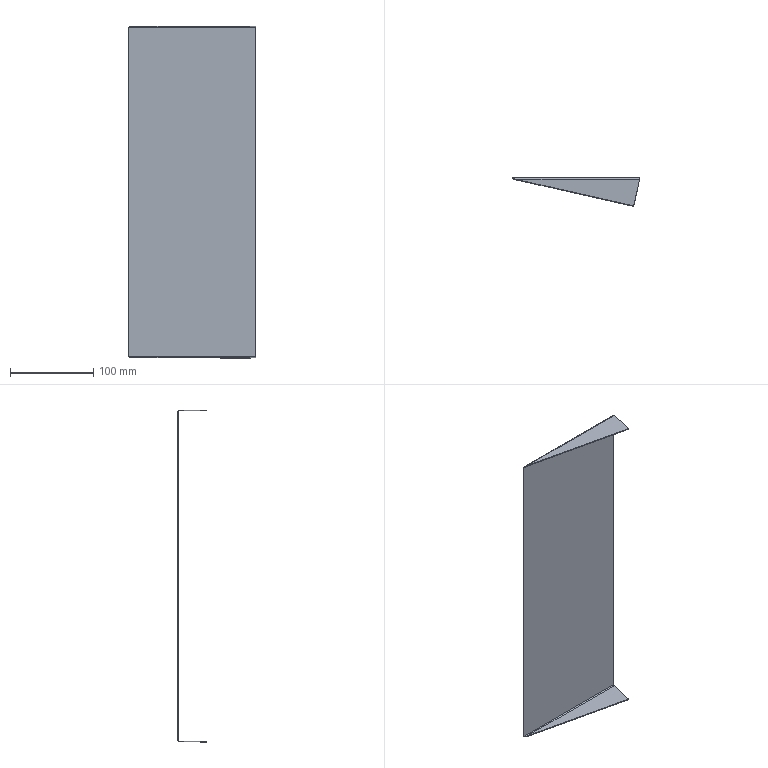Part | SolidWorks | features EdgeFlange 1, FlatPattern 1, MirrorPattern 1, SMBaseFlange 1, SheetMetal 1 | 1 solid | 20 faces | box 153.5 x 34 x 399 mm | volume 66108 mm3 | plane 12 | spline 4 | cylinder 4 | commonest cylinder face diameters 2 x2 4 x2
STEP:
#1=CARTESIAN_POINT('',(0.,-1.,-197.5));
#2=VERTEX_POINT('',#1);
#3=CARTESIAN_POINT('',(-153.5,-1.,-197.5));
#4=VERTEX_POINT('',#3);
#5=CARTESIAN_POINT('',(0.,-1.,-197.5));
#6=DIRECTION('',(-1.,0.,0.));
#7=VECTOR('',#6,1000.);
#8=LINE('',#5,#7);
#9=EDGE_CURVE('',#2,#4,#8,.T.);
#10=ORIENTED_EDGE('',*,*,#9,.F.);
#11=CARTESIAN_POINT('',(0.,-1.,197.5));
#12=VERTEX_POINT('',#11);
#13=CARTESIAN_POINT('',(0.,-1.,199.5));
#14=DIRECTION('',(0.,0.,-1.));
#15=VECTOR('',#14,1000.);
#16=LINE('',#13,#15);
#17=EDGE_CURVE('',#12,#2,#16,.T.);
#18=ORIENTED_EDGE('',*,*,#17,.F.);
#19=CARTESIAN_POINT('',(-153.5,-1.,197.5));
#20=VERTEX_POINT('',#19);
#21=CARTESIAN_POINT('',(-153.5,-1.,197.5));
#22=DIRECTION('',(1.,0.,0.));
#23=VECTOR('',#22,1000.);
#24=LINE('',#21,#23);
#25=EDGE_CURVE('',#20,#12,#24,.T.);
#26=ORIENTED_EDGE('',*,*,#25,.F.);
#27=CARTESIAN_POINT('',(-153.5,-1.,199.5));
#28=DIRECTION('',(0.,0.,-1.));
#29=VECTOR('',#28,1000.);
#30=LINE('',#27,#29);
#31=EDGE_CURVE('',#20,#4,#30,.T.);
#32=ORIENTED_EDGE('',*,*,#31,.T.);
#33=EDGE_LOOP('',(#10,#18,#26,#32));
#34=FACE_OUTER_BOUND('',#33,.T.);
#35=CARTESIAN_POINT('',(-153.5,-1.,199.5));
#36=DIRECTION('',(0.,1.,0.));
#37=DIRECTION('',(0.,0.,1.));
#38=AXIS2_PLACEMENT_3D('',#35,#36,#37);
#39=PLANE('',#38);
#40=ADVANCED_FACE('',(#34),#39,.F.);
#41=CARTESIAN_POINT('',(0.,0.,197.5));
#42=VERTEX_POINT('',#41);
#43=CARTESIAN_POINT('',(0.,0.,-197.5));
#44=VERTEX_POINT('',#43);
#45=CARTESIAN_POINT('',(0.,0.,199.5));
#46=DIRECTION('',(0.,0.,-1.));
#47=VECTOR('',#46,1000.);
#48=LINE('',#45,#47);
#49=EDGE_CURVE('',#42,#44,#48,.T.);
#50=ORIENTED_EDGE('',*,*,#49,.T.);
#51=CARTESIAN_POINT('',(-153.5,0.,-197.5));
#52=VERTEX_POINT('',#51);
#53=CARTESIAN_POINT('',(0.,0.,-197.5));
#54=DIRECTION('',(-1.,0.,0.));
#55=VECTOR('',#54,1000.);
#56=LINE('',#53,#55);
#57=EDGE_CURVE('',#44,#52,#56,.T.);
#58=ORIENTED_EDGE('',*,*,#57,.T.);
#59=CARTESIAN_POINT('',(-153.5,0.,197.5));
#60=VERTEX_POINT('',#59);
#61=CARTESIAN_POINT('',(-153.5,0.,199.5));
#62=DIRECTION('',(0.,0.,-1.));
#63=VECTOR('',#62,1000.);
#64=LINE('',#61,#63);
#65=EDGE_CURVE('',#60,#52,#64,.T.);
#66=ORIENTED_EDGE('',*,*,#65,.F.);
#67=CARTESIAN_POINT('',(-153.5,0.,197.5));
#68=DIRECTION('',(1.,0.,0.));
#69=VECTOR('',#68,1000.);
#70=LINE('',#67,#69);
#71=EDGE_CURVE('',#60,#42,#70,.T.);
#72=ORIENTED_EDGE('',*,*,#71,.T.);
#73=EDGE_LOOP('',(#50,#58,#66,#72));
#74=FACE_OUTER_BOUND('',#73,.T.);
#75=CARTESIAN_POINT('',(-153.5,0.,199.5));
#76=DIRECTION('',(0.,1.,0.));
#77=DIRECTION('',(0.,0.,1.));
#78=AXIS2_PLACEMENT_3D('',#75,#76,#77);
#79=PLANE('',#78);
#80=ADVANCED_FACE('',(#74),#79,.T.);
#81=ORIENTED_EDGE('',*,*,#17,.T.);
#82=CARTESIAN_POINT('',(0.,-1.,-197.5));
#83=DIRECTION('',(0.,1.,0.));
#84=VECTOR('',#83,1000.);
#85=LINE('',#82,#84);
#86=EDGE_CURVE('',#2,#44,#85,.T.);
#87=ORIENTED_EDGE('',*,*,#86,.T.);
#88=ORIENTED_EDGE('',*,*,#49,.F.);
#89=CARTESIAN_POINT('',(0.,-1.,197.5));
#90=DIRECTION('',(0.,1.,0.));
#91=VECTOR('',#90,1000.);
#92=LINE('',#89,#91);
#93=EDGE_CURVE('',#12,#42,#92,.T.);
#94=ORIENTED_EDGE('',*,*,#93,.F.);
#95=EDGE_LOOP('',(#81,#87,#88,#94));
#96=FACE_OUTER_BOUND('',#95,.T.);
#97=CARTESIAN_POINT('',(0.,0.,199.5));
#98=DIRECTION('',(1.,0.,0.));
#99=DIRECTION('',(0.,0.,-1.));
#100=AXIS2_PLACEMENT_3D('',#97,#98,#99);
#101=PLANE('',#100);
#102=ADVANCED_FACE('',(#96),#101,.T.);
#103=CARTESIAN_POINT('',(-153.5,-1.,-197.5));
#104=DIRECTION('',(0.,1.,0.));
#105=VECTOR('',#104,1000.);
#106=LINE('',#103,#105);
#107=EDGE_CURVE('',#4,#52,#106,.T.);
#108=ORIENTED_EDGE('',*,*,#107,.F.);
#109=ORIENTED_EDGE('',*,*,#31,.F.);
#110=CARTESIAN_POINT('',(-153.5,-1.,197.5));
#111=DIRECTION('',(0.,1.,0.));
#112=VECTOR('',#111,1000.);
#113=LINE('',#110,#112);
#114=EDGE_CURVE('',#20,#60,#113,.T.);
#115=ORIENTED_EDGE('',*,*,#114,.T.);
#116=ORIENTED_EDGE('',*,*,#65,.T.);
#117=EDGE_LOOP('',(#108,#109,#115,#116));
#118=FACE_OUTER_BOUND('',#117,.T.);
#119=CARTESIAN_POINT('',(-153.5,-1.,199.5));
#120=DIRECTION('',(-1.,0.,0.));
#121=DIRECTION('',(0.,0.,1.));
#122=AXIS2_PLACEMENT_3D('',#119,#120,#121);
#123=PLANE('',#122);
#124=ADVANCED_FACE('',(#118),#123,.T.);
#125=CARTESIAN_POINT('',(-0.226,-2.,198.5));
#126=VERTEX_POINT('',#125);
#127=CARTESIAN_POINT('',(-0.226,-2.,199.5));
#128=VERTEX_POINT('',#127);
#129=CARTESIAN_POINT('',(-0.226,-2.,199.5));
#130=DIRECTION('',(0.,0.,1.));
#131=VECTOR('',#130,1000.);
#132=LINE('',#129,#131);
#133=EDGE_CURVE('',#126,#128,#132,.T.);
#134=ORIENTED_EDGE('',*,*,#133,.F.);
#135=CARTESIAN_POINT('',(0.,-1.,197.5));
#136=CARTESIAN_POINT('',(-0.03766,-1.,197.762));
#137=CARTESIAN_POINT('',(-0.07532,-1.108,198.022));
#138=CARTESIAN_POINT('',(-0.1506,-1.478,198.392));
#139=CARTESIAN_POINT('',(-0.1883,-1.738,198.5));
#140=CARTESIAN_POINT('',(-0.226,-2.,198.5));
#141=B_SPLINE_CURVE_WITH_KNOTS('',3,(#135,#136,#137,#138,#139,#140),.UNSPECIFIED.,.F.,.F.,(4,2,4),(0.,0.5,1.),.UNSPECIFIED.);
#142=EDGE_CURVE('',#12,#126,#141,.T.);
#143=ORIENTED_EDGE('',*,*,#142,.F.);
#144=ORIENTED_EDGE('',*,*,#93,.T.);
#145=CARTESIAN_POINT('',(0.,0.,197.5));
#146=CARTESIAN_POINT('',(-0.01883,0.,197.762));
#147=CARTESIAN_POINT('',(-0.03766,-0.05205,198.023));
#148=CARTESIAN_POINT('',(-0.07532,-0.2524,198.507));
#149=CARTESIAN_POINT('',(-0.09415,-0.4007,198.729));
#150=CARTESIAN_POINT('',(-0.1318,-0.7709,199.099));
#151=CARTESIAN_POINT('',(-0.1506,-0.9928,199.248));
#152=CARTESIAN_POINT('',(-0.1883,-1.477,199.448));
#153=CARTESIAN_POINT('',(-0.2071,-1.738,199.5));
#154=CARTESIAN_POINT('',(-0.226,-2.,199.5));
#155=B_SPLINE_CURVE_WITH_KNOTS('',3,(#145,#146,#147,#148,#149,#150,#151,#152,#153,#154),.UNSPECIFIED.,.F.,.F.,(4,2,2,2,4),(0.,0.25,0.5,0.75,1.),.UNSPECIFIED.);
#156=EDGE_CURVE('',#42,#128,#155,.T.);
#157=ORIENTED_EDGE('',*,*,#156,.T.);
#158=EDGE_LOOP('',(#134,#143,#144,#157));
#159=FACE_OUTER_BOUND('',#158,.T.);
#160=CARTESIAN_POINT('',(0.,0.01,197.5));
#161=CARTESIAN_POINT('',(-0.01883,0.01,197.763));
#162=CARTESIAN_POINT('',(-0.03766,-0.04231,198.026));
#163=CARTESIAN_POINT('',(-0.07532,-0.2437,198.512));
#164=CARTESIAN_POINT('',(-0.09415,-0.3927,198.735));
#165=CARTESIAN_POINT('',(-0.1318,-0.7648,199.107));
#166=CARTESIAN_POINT('',(-0.1506,-0.9877,199.256));
#167=CARTESIAN_POINT('',(-0.1883,-1.474,199.458));
#168=CARTESIAN_POINT('',(-0.2071,-1.737,199.51));
#169=CARTESIAN_POINT('',(-0.226,-2.,199.51));
#170=CARTESIAN_POINT('',(0.,0.,197.5));
#171=CARTESIAN_POINT('',(-0.01883,0.,197.762));
#172=CARTESIAN_POINT('',(-0.03766,-0.05205,198.023));
#173=CARTESIAN_POINT('',(-0.07532,-0.2524,198.507));
#174=CARTESIAN_POINT('',(-0.09415,-0.4007,198.729));
#175=CARTESIAN_POINT('',(-0.1318,-0.7709,199.099));
#176=CARTESIAN_POINT('',(-0.1506,-0.9928,199.248));
#177=CARTESIAN_POINT('',(-0.1883,-1.477,199.448));
#178=CARTESIAN_POINT('',(-0.2071,-1.738,199.5));
#179=CARTESIAN_POINT('',(-0.226,-2.,199.5));
#180=CARTESIAN_POINT('',(0.,-1.,197.5));
#181=CARTESIAN_POINT('',(-0.01883,-1.,197.631));
#182=CARTESIAN_POINT('',(-0.03766,-1.026,197.762));
#183=CARTESIAN_POINT('',(-0.07532,-1.126,198.004));
#184=CARTESIAN_POINT('',(-0.09415,-1.2,198.115));
#185=CARTESIAN_POINT('',(-0.1318,-1.385,198.3));
#186=CARTESIAN_POINT('',(-0.1506,-1.496,198.374));
#187=CARTESIAN_POINT('',(-0.1883,-1.738,198.474));
#188=CARTESIAN_POINT('',(-0.2071,-1.869,198.5));
#189=CARTESIAN_POINT('',(-0.226,-2.,198.5));
#190=CARTESIAN_POINT('',(0.,-1.01,197.5));
#191=CARTESIAN_POINT('',(-0.01883,-1.01,197.63));
#192=CARTESIAN_POINT('',(-0.03766,-1.036,197.759));
#193=CARTESIAN_POINT('',(-0.07532,-1.135,197.999));
#194=CARTESIAN_POINT('',(-0.09415,-1.208,198.108));
#195=CARTESIAN_POINT('',(-0.1318,-1.392,198.292));
#196=CARTESIAN_POINT('',(-0.1506,-1.501,198.365));
#197=CARTESIAN_POINT('',(-0.1883,-1.741,198.464));
#198=CARTESIAN_POINT('',(-0.2071,-1.87,198.49));
#199=CARTESIAN_POINT('',(-0.226,-2.,198.49));
#200=B_SPLINE_SURFACE_WITH_KNOTS('',1,3,((#160,#161,#162,#163,#164,#165,#166,#167,#168,#169),(#170,#171,#172,#173,#174,#175,#176,#177,#178,#179),(#180,#181,#182,#183,#184,#185,#186,#187,#188,#189),(#190,#191,#192,#193,#194,#195,#196,#197,#198,#199)),.UNSPECIFIED.,.F.,.F.,.F.,(2,1,1,2),(4,2,2,2,4),(-0.01,0.,1.,1.01),(0.,0.25,0.5,0.75,1.),.UNSPECIFIED.);
#201=ADVANCED_FACE('',(#159),#200,.F.);
#202=CARTESIAN_POINT('',(-149.074,-2.,198.5));
#203=VERTEX_POINT('',#202);
#204=CARTESIAN_POINT('',(-149.074,-2.,198.5));
#205=CARTESIAN_POINT('',(-149.444,-1.869,198.5));
#206=CARTESIAN_POINT('',(-149.811,-1.738,198.474));
#207=CARTESIAN_POINT('',(-150.547,-1.497,198.374));
#208=CARTESIAN_POINT('',(-150.916,-1.386,198.3));
#209=CARTESIAN_POINT('',(-151.654,-1.201,198.115));
#210=CARTESIAN_POINT('',(-152.023,-1.126,198.004));
#211=CARTESIAN_POINT('',(-152.762,-1.026,197.762));
#212=CARTESIAN_POINT('',(-153.13,-1.,197.631));
#213=CARTESIAN_POINT('',(-153.5,-1.,197.5));
#214=B_SPLINE_CURVE_WITH_KNOTS('',3,(#204,#205,#206,#207,#208,#209,#210,#211,#212,#213),.UNSPECIFIED.,.F.,.F.,(4,2,2,2,4),(0.,0.00117,0.00234,0.00351,0.00468),.UNSPECIFIED.);
#215=EDGE_CURVE('',#203,#20,#214,.T.);
#216=ORIENTED_EDGE('',*,*,#215,.F.);
#217=CARTESIAN_POINT('',(-149.074,-2.,199.5));
#218=VERTEX_POINT('',#217);
#219=CARTESIAN_POINT('',(-149.074,-2.,198.5));
#220=DIRECTION('',(0.,0.,1.));
#221=VECTOR('',#220,1000.);
#222=LINE('',#219,#221);
#223=EDGE_CURVE('',#203,#218,#222,.T.);
#224=ORIENTED_EDGE('',*,*,#223,.T.);
#225=CARTESIAN_POINT('',(-149.074,-2.,199.5));
#226=CARTESIAN_POINT('',(-149.446,-1.736,199.5));
#227=CARTESIAN_POINT('',(-149.811,-1.477,199.448));
#228=CARTESIAN_POINT('',(-150.545,-0.9954,199.249));
#229=CARTESIAN_POINT('',(-150.918,-0.771,199.099));
#230=CARTESIAN_POINT('',(-151.653,-0.4023,198.731));
#231=CARTESIAN_POINT('',(-152.018,-0.2546,198.512));
#232=CARTESIAN_POINT('',(-152.761,-0.05202,198.024));
#233=CARTESIAN_POINT('',(-153.128,0.,197.764));
#234=CARTESIAN_POINT('',(-153.5,0.,197.5));
#235=B_SPLINE_CURVE_WITH_KNOTS('',3,(#225,#226,#227,#228,#229,#230,#231,#232,#233,#234),.UNSPECIFIED.,.F.,.F.,(4,2,2,2,4),(0.,0.001349,0.002697,0.004046,0.005395),.UNSPECIFIED.);
#236=EDGE_CURVE('',#218,#60,#235,.T.);
#237=ORIENTED_EDGE('',*,*,#236,.T.);
#238=ORIENTED_EDGE('',*,*,#114,.F.);
#239=EDGE_LOOP('',(#216,#224,#237,#238));
#240=FACE_OUTER_BOUND('',#239,.T.);
#241=CARTESIAN_POINT('',(-149.074,-2.,199.51));
#242=CARTESIAN_POINT('',(-149.443,-1.737,199.51));
#243=CARTESIAN_POINT('',(-149.812,-1.474,199.458));
#244=CARTESIAN_POINT('',(-150.55,-0.9877,199.256));
#245=CARTESIAN_POINT('',(-150.918,-0.7648,199.107));
#246=CARTESIAN_POINT('',(-151.656,-0.3927,198.735));
#247=CARTESIAN_POINT('',(-152.025,-0.2437,198.512));
#248=CARTESIAN_POINT('',(-152.762,-0.04231,198.026));
#249=CARTESIAN_POINT('',(-153.131,0.01,197.763));
#250=CARTESIAN_POINT('',(-153.5,0.01,197.5));
#251=CARTESIAN_POINT('',(-149.074,-2.,199.5));
#252=CARTESIAN_POINT('',(-149.443,-1.738,199.5));
#253=CARTESIAN_POINT('',(-149.812,-1.477,199.448));
#254=CARTESIAN_POINT('',(-150.55,-0.9928,199.248));
#255=CARTESIAN_POINT('',(-150.918,-0.7709,199.099));
#256=CARTESIAN_POINT('',(-151.656,-0.4007,198.729));
#257=CARTESIAN_POINT('',(-152.025,-0.2524,198.507));
#258=CARTESIAN_POINT('',(-152.762,-0.05205,198.023));
#259=CARTESIAN_POINT('',(-153.131,0.,197.762));
#260=CARTESIAN_POINT('',(-153.5,0.,197.5));
#261=CARTESIAN_POINT('',(-149.074,-2.,198.5));
#262=CARTESIAN_POINT('',(-149.443,-1.869,198.5));
#263=CARTESIAN_POINT('',(-149.812,-1.738,198.474));
#264=CARTESIAN_POINT('',(-150.55,-1.496,198.374));
#265=CARTESIAN_POINT('',(-150.918,-1.385,198.3));
#266=CARTESIAN_POINT('',(-151.656,-1.2,198.115));
#267=CARTESIAN_POINT('',(-152.025,-1.126,198.004));
#268=CARTESIAN_POINT('',(-152.762,-1.026,197.762));
#269=CARTESIAN_POINT('',(-153.131,-1.,197.631));
#270=CARTESIAN_POINT('',(-153.5,-1.,197.5));
#271=CARTESIAN_POINT('',(-149.074,-2.,198.49));
#272=CARTESIAN_POINT('',(-149.443,-1.87,198.49));
#273=CARTESIAN_POINT('',(-149.812,-1.741,198.464));
#274=CARTESIAN_POINT('',(-150.55,-1.501,198.365));
#275=CARTESIAN_POINT('',(-150.918,-1.392,198.292));
#276=CARTESIAN_POINT('',(-151.656,-1.208,198.108));
#277=CARTESIAN_POINT('',(-152.025,-1.135,197.999));
#278=CARTESIAN_POINT('',(-152.762,-1.036,197.759));
#279=CARTESIAN_POINT('',(-153.131,-1.01,197.63));
#280=CARTESIAN_POINT('',(-153.5,-1.01,197.5));
#281=B_SPLINE_SURFACE_WITH_KNOTS('',1,3,((#241,#242,#243,#244,#245,#246,#247,#248,#249,#250),(#251,#252,#253,#254,#255,#256,#257,#258,#259,#260),(#261,#262,#263,#264,#265,#266,#267,#268,#269,#270),(#271,#272,#273,#274,#275,#276,#277,#278,#279,#280)),.UNSPECIFIED.,.F.,.F.,.F.,(2,1,1,2),(4,2,2,2,4),(-0.01,0.,1.,1.01),(0.,0.25,0.5,0.75,1.),.UNSPECIFIED.);
#282=ADVANCED_FACE('',(#240),#281,.F.);
#283=ORIENTED_EDGE('',*,*,#71,.F.);
#284=ORIENTED_EDGE('',*,*,#236,.F.);
#285=CARTESIAN_POINT('',(-0.226,-2.,199.5));
#286=DIRECTION('',(1.,0.,0.));
#287=VECTOR('',#286,1000.);
#288=LINE('',#285,#287);
#289=EDGE_CURVE('',#218,#128,#288,.T.);
#290=ORIENTED_EDGE('',*,*,#289,.T.);
#291=ORIENTED_EDGE('',*,*,#156,.F.);
#292=EDGE_LOOP('',(#283,#284,#290,#291));
#293=FACE_OUTER_BOUND('',#292,.T.);
#294=CARTESIAN_POINT('',(-153.5,-2.,197.5));
#295=DIRECTION('',(-1.,0.,0.));
#296=DIRECTION('',(0.,0.,1.));
#297=AXIS2_PLACEMENT_3D('',#294,#295,#296);
#298=CYLINDRICAL_SURFACE('',#297,2.);
#299=ADVANCED_FACE('',(#293),#298,.T.);
#300=ORIENTED_EDGE('',*,*,#25,.T.);
#301=ORIENTED_EDGE('',*,*,#142,.T.);
#302=CARTESIAN_POINT('',(-0.226,-2.,198.5));
#303=DIRECTION('',(-1.,0.,0.));
#304=VECTOR('',#303,1000.);
#305=LINE('',#302,#304);
#306=EDGE_CURVE('',#126,#203,#305,.T.);
#307=ORIENTED_EDGE('',*,*,#306,.T.);
#308=ORIENTED_EDGE('',*,*,#215,.T.);
#309=EDGE_LOOP('',(#300,#301,#307,#308));
#310=FACE_OUTER_BOUND('',#309,.T.);
#311=CARTESIAN_POINT('',(-153.5,-2.,197.5));
#312=DIRECTION('',(-1.,0.,0.));
#313=DIRECTION('',(0.,0.,1.));
#314=AXIS2_PLACEMENT_3D('',#311,#312,#313);
#315=CYLINDRICAL_SURFACE('',#314,1.);
#316=ADVANCED_FACE('',(#310),#315,.F.);
#317=CARTESIAN_POINT('',(-7.457,-34.,199.5));
#318=VERTEX_POINT('',#317);
#319=CARTESIAN_POINT('',(-153.5,-1.,199.5));
#320=DIRECTION('',(-0.9754,0.2204,0.));
#321=VECTOR('',#320,1000.);
#322=LINE('',#319,#321);
#323=EDGE_CURVE('',#318,#218,#322,.T.);
#324=ORIENTED_EDGE('',*,*,#323,.T.);
#325=ORIENTED_EDGE('',*,*,#223,.F.);
#326=CARTESIAN_POINT('',(-7.457,-34.,198.5));
#327=VERTEX_POINT('',#326);
#328=CARTESIAN_POINT('',(-7.672,-33.951,198.5));
#329=DIRECTION('',(-0.9754,0.2204,0.));
#330=VECTOR('',#329,1000.);
#331=LINE('',#328,#330);
#332=EDGE_CURVE('',#327,#203,#331,.T.);
#333=ORIENTED_EDGE('',*,*,#332,.F.);
#334=CARTESIAN_POINT('',(-7.457,-34.,199.5));
#335=DIRECTION('',(0.,0.,-1.));
#336=VECTOR('',#335,1000.);
#337=LINE('',#334,#336);
#338=EDGE_CURVE('',#318,#327,#337,.T.);
#339=ORIENTED_EDGE('',*,*,#338,.F.);
#340=EDGE_LOOP('',(#324,#325,#333,#339));
#341=FACE_OUTER_BOUND('',#340,.T.);
#342=CARTESIAN_POINT('',(-153.5,-1.,199.5));
#343=DIRECTION('',(-0.2204,-0.9754,0.));
#344=DIRECTION('',(0.9754,-0.2204,0.));
#345=AXIS2_PLACEMENT_3D('',#342,#343,#344);
#346=PLANE('',#345);
#347=ADVANCED_FACE('',(#341),#346,.T.);
#348=CARTESIAN_POINT('',(0.215,-0.04858,198.5));
#349=DIRECTION('',(-0.2204,-0.9754,0.));
#350=VECTOR('',#349,1000.);
#351=LINE('',#348,#350);
#352=EDGE_CURVE('',#126,#327,#351,.T.);
#353=ORIENTED_EDGE('',*,*,#352,.F.);
#354=ORIENTED_EDGE('',*,*,#133,.T.);
#355=CARTESIAN_POINT('',(-7.457,-34.,199.5));
#356=DIRECTION('',(-0.2204,-0.9754,0.));
#357=VECTOR('',#356,1000.);
#358=LINE('',#355,#357);
#359=EDGE_CURVE('',#128,#318,#358,.T.);
#360=ORIENTED_EDGE('',*,*,#359,.T.);
#361=ORIENTED_EDGE('',*,*,#338,.T.);
#362=EDGE_LOOP('',(#353,#354,#360,#361));
#363=FACE_OUTER_BOUND('',#362,.T.);
#364=CARTESIAN_POINT('',(-7.457,-34.,199.5));
#365=DIRECTION('',(0.9754,-0.2204,0.));
#366=DIRECTION('',(0.2204,0.9754,0.));
#367=AXIS2_PLACEMENT_3D('',#364,#365,#366);
#368=PLANE('',#367);
#369=ADVANCED_FACE('',(#363),#368,.T.);
#370=ORIENTED_EDGE('',*,*,#289,.F.);
#371=ORIENTED_EDGE('',*,*,#323,.F.);
#372=ORIENTED_EDGE('',*,*,#359,.F.);
#373=EDGE_LOOP('',(#370,#371,#372));
#374=FACE_OUTER_BOUND('',#373,.T.);
#375=CARTESIAN_POINT('',(0.,0.,199.5));
#376=DIRECTION('',(0.,0.,-1.));
#377=DIRECTION('',(0.,1.,0.));
#378=AXIS2_PLACEMENT_3D('',#375,#376,#377);
#379=PLANE('',#378);
#380=ADVANCED_FACE('',(#374),#379,.F.);
#381=ORIENTED_EDGE('',*,*,#332,.T.);
#382=ORIENTED_EDGE('',*,*,#306,.F.);
#383=ORIENTED_EDGE('',*,*,#352,.T.);
#384=EDGE_LOOP('',(#381,#382,#383));
#385=FACE_OUTER_BOUND('',#384,.T.);
#386=CARTESIAN_POINT('',(0.,0.,198.5));
#387=DIRECTION('',(0.,0.,-1.));
#388=DIRECTION('',(0.,1.,0.));
#389=AXIS2_PLACEMENT_3D('',#386,#387,#388);
#390=PLANE('',#389);
#391=ADVANCED_FACE('',(#385),#390,.T.);
#392=CARTESIAN_POINT('',(-149.074,-2.,-198.5));
#393=VERTEX_POINT('',#392);
#394=CARTESIAN_POINT('',(-149.074,-2.,-199.5));
#395=VERTEX_POINT('',#394);
#396=CARTESIAN_POINT('',(-149.074,-2.,-199.5));
#397=DIRECTION('',(0.,0.,-1.));
#398=VECTOR('',#397,1000.);
#399=LINE('',#396,#398);
#400=EDGE_CURVE('',#393,#395,#399,.T.);
#401=ORIENTED_EDGE('',*,*,#400,.F.);
#402=CARTESIAN_POINT('',(-153.5,-1.,-197.5));
#403=CARTESIAN_POINT('',(-153.13,-1.,-197.631));
#404=CARTESIAN_POINT('',(-152.763,-1.026,-197.762));
#405=CARTESIAN_POINT('',(-152.028,-1.126,-198.003));
#406=CARTESIAN_POINT('',(-151.658,-1.2,-198.114));
#407=CARTESIAN_POINT('',(-150.92,-1.385,-198.299));
#408=CARTESIAN_POINT('',(-150.551,-1.496,-198.374));
#409=CARTESIAN_POINT('',(-149.812,-1.738,-198.474));
#410=CARTESIAN_POINT('',(-149.444,-1.869,-198.5));
#411=CARTESIAN_POINT('',(-149.074,-2.,-198.5));
#412=B_SPLINE_CURVE_WITH_KNOTS('',3,(#402,#403,#404,#405,#406,#407,#408,#409,#410,#411),.UNSPECIFIED.,.F.,.F.,(4,2,2,2,4),(0.,0.00117,0.00234,0.00351,0.00468),.UNSPECIFIED.);
#413=EDGE_CURVE('',#4,#393,#412,.T.);
#414=ORIENTED_EDGE('',*,*,#413,.F.);
#415=ORIENTED_EDGE('',*,*,#107,.T.);
#416=CARTESIAN_POINT('',(-153.5,0.,-197.5));
#417=CARTESIAN_POINT('',(-153.128,0.,-197.764));
#418=CARTESIAN_POINT('',(-152.763,-0.05201,-198.023));
#419=CARTESIAN_POINT('',(-152.029,-0.2511,-198.505));
#420=CARTESIAN_POINT('',(-151.656,-0.4008,-198.729));
#421=CARTESIAN_POINT('',(-150.922,-0.7691,-199.098));
#422=CARTESIAN_POINT('',(-150.556,-0.9885,-199.245));
#423=CARTESIAN_POINT('',(-149.813,-1.476,-199.448));
#424=CARTESIAN_POINT('',(-149.446,-1.736,-199.5));
#425=CARTESIAN_POINT('',(-149.074,-2.,-199.5));
#426=B_SPLINE_CURVE_WITH_KNOTS('',3,(#416,#417,#418,#419,#420,#421,#422,#423,#424,#425),.UNSPECIFIED.,.F.,.F.,(4,2,2,2,4),(0.,0.001349,0.002697,0.004046,0.005395),.UNSPECIFIED.);
#427=EDGE_CURVE('',#52,#395,#426,.T.);
#428=ORIENTED_EDGE('',*,*,#427,.T.);
#429=EDGE_LOOP('',(#401,#414,#415,#428));
#430=FACE_OUTER_BOUND('',#429,.T.);
#431=CARTESIAN_POINT('',(-153.5,0.01,-197.5));
#432=CARTESIAN_POINT('',(-153.131,0.01,-197.763));
#433=CARTESIAN_POINT('',(-152.762,-0.04231,-198.026));
#434=CARTESIAN_POINT('',(-152.025,-0.2437,-198.512));
#435=CARTESIAN_POINT('',(-151.656,-0.3927,-198.735));
#436=CARTESIAN_POINT('',(-150.918,-0.7648,-199.107));
#437=CARTESIAN_POINT('',(-150.55,-0.9877,-199.256));
#438=CARTESIAN_POINT('',(-149.812,-1.474,-199.458));
#439=CARTESIAN_POINT('',(-149.443,-1.737,-199.51));
#440=CARTESIAN_POINT('',(-149.074,-2.,-199.51));
#441=CARTESIAN_POINT('',(-153.5,0.,-197.5));
#442=CARTESIAN_POINT('',(-153.131,0.,-197.762));
#443=CARTESIAN_POINT('',(-152.762,-0.05205,-198.023));
#444=CARTESIAN_POINT('',(-152.025,-0.2524,-198.507));
#445=CARTESIAN_POINT('',(-151.656,-0.4007,-198.729));
#446=CARTESIAN_POINT('',(-150.918,-0.7709,-199.099));
#447=CARTESIAN_POINT('',(-150.55,-0.9928,-199.248));
#448=CARTESIAN_POINT('',(-149.812,-1.477,-199.448));
#449=CARTESIAN_POINT('',(-149.443,-1.738,-199.5));
#450=CARTESIAN_POINT('',(-149.074,-2.,-199.5));
#451=CARTESIAN_POINT('',(-153.5,-1.,-197.5));
#452=CARTESIAN_POINT('',(-153.131,-1.,-197.631));
#453=CARTESIAN_POINT('',(-152.762,-1.026,-197.762));
#454=CARTESIAN_POINT('',(-152.025,-1.126,-198.004));
#455=CARTESIAN_POINT('',(-151.656,-1.2,-198.115));
#456=CARTESIAN_POINT('',(-150.918,-1.385,-198.3));
#457=CARTESIAN_POINT('',(-150.55,-1.496,-198.374));
#458=CARTESIAN_POINT('',(-149.812,-1.738,-198.474));
#459=CARTESIAN_POINT('',(-149.443,-1.869,-198.5));
#460=CARTESIAN_POINT('',(-149.074,-2.,-198.5));
#461=CARTESIAN_POINT('',(-153.5,-1.01,-197.5));
#462=CARTESIAN_POINT('',(-153.131,-1.01,-197.63));
#463=CARTESIAN_POINT('',(-152.762,-1.036,-197.759));
#464=CARTESIAN_POINT('',(-152.025,-1.135,-197.999));
#465=CARTESIAN_POINT('',(-151.656,-1.208,-198.108));
#466=CARTESIAN_POINT('',(-150.918,-1.392,-198.292));
#467=CARTESIAN_POINT('',(-150.55,-1.501,-198.365));
#468=CARTESIAN_POINT('',(-149.812,-1.741,-198.464));
#469=CARTESIAN_POINT('',(-149.443,-1.87,-198.49));
#470=CARTESIAN_POINT('',(-149.074,-2.,-198.49));
#471=B_SPLINE_SURFACE_WITH_KNOTS('',1,3,((#431,#432,#433,#434,#435,#436,#437,#438,#439,#440),(#441,#442,#443,#444,#445,#446,#447,#448,#449,#450),(#451,#452,#453,#454,#455,#456,#457,#458,#459,#460),(#461,#462,#463,#464,#465,#466,#467,#468,#469,#470)),.UNSPECIFIED.,.F.,.F.,.F.,(2,1,1,2),(4,2,2,2,4),(-0.01,0.,1.,1.01),(0.,0.25,0.5,0.75,1.),.UNSPECIFIED.);
#472=ADVANCED_FACE('',(#430),#471,.F.);
#473=CARTESIAN_POINT('',(-0.226,-2.,-198.5));
#474=VERTEX_POINT('',#473);
#475=CARTESIAN_POINT('',(-0.226,-2.,-198.5));
#476=CARTESIAN_POINT('',(-0.1883,-1.738,-198.5));
#477=CARTESIAN_POINT('',(-0.1506,-1.478,-198.392));
#478=CARTESIAN_POINT('',(-0.07532,-1.108,-198.022));
#479=CARTESIAN_POINT('',(-0.03766,-1.,-197.762));
#480=CARTESIAN_POINT('',(0.,-1.,-197.5));
#481=B_SPLINE_CURVE_WITH_KNOTS('',3,(#475,#476,#477,#478,#479,#480),.UNSPECIFIED.,.F.,.F.,(4,2,4),(0.,0.5,1.),.UNSPECIFIED.);
#482=EDGE_CURVE('',#474,#2,#481,.T.);
#483=ORIENTED_EDGE('',*,*,#482,.F.);
#484=CARTESIAN_POINT('',(-0.226,-2.,-199.5));
#485=VERTEX_POINT('',#484);
#486=CARTESIAN_POINT('',(-0.226,-2.,-198.5));
#487=DIRECTION('',(0.,0.,-1.));
#488=VECTOR('',#487,1000.);
#489=LINE('',#486,#488);
#490=EDGE_CURVE('',#474,#485,#489,.T.);
#491=ORIENTED_EDGE('',*,*,#490,.T.);
#492=CARTESIAN_POINT('',(-0.226,-2.,-199.5));
#493=CARTESIAN_POINT('',(-0.2071,-1.738,-199.5));
#494=CARTESIAN_POINT('',(-0.1883,-1.477,-199.448));
#495=CARTESIAN_POINT('',(-0.1506,-0.9928,-199.248));
#496=CARTESIAN_POINT('',(-0.1318,-0.7709,-199.099));
#497=CARTESIAN_POINT('',(-0.09415,-0.4007,-198.729));
#498=CARTESIAN_POINT('',(-0.07532,-0.2524,-198.507));
#499=CARTESIAN_POINT('',(-0.03766,-0.05205,-198.023));
#500=CARTESIAN_POINT('',(-0.01883,0.,-197.762));
#501=CARTESIAN_POINT('',(0.,0.,-197.5));
#502=B_SPLINE_CURVE_WITH_KNOTS('',3,(#492,#493,#494,#495,#496,#497,#498,#499,#500,#501),.UNSPECIFIED.,.F.,.F.,(4,2,2,2,4),(0.,0.25,0.5,0.75,1.),.UNSPECIFIED.);
#503=EDGE_CURVE('',#485,#44,#502,.T.);
#504=ORIENTED_EDGE('',*,*,#503,.T.);
#505=ORIENTED_EDGE('',*,*,#86,.F.);
#506=EDGE_LOOP('',(#483,#491,#504,#505));
#507=FACE_OUTER_BOUND('',#506,.T.);
#508=CARTESIAN_POINT('',(-0.226,-2.,-199.51));
#509=CARTESIAN_POINT('',(-0.2071,-1.737,-199.51));
#510=CARTESIAN_POINT('',(-0.1883,-1.474,-199.458));
#511=CARTESIAN_POINT('',(-0.1506,-0.9877,-199.256));
#512=CARTESIAN_POINT('',(-0.1318,-0.7648,-199.107));
#513=CARTESIAN_POINT('',(-0.09415,-0.3927,-198.735));
#514=CARTESIAN_POINT('',(-0.07532,-0.2437,-198.512));
#515=CARTESIAN_POINT('',(-0.03766,-0.04231,-198.026));
#516=CARTESIAN_POINT('',(-0.01883,0.01,-197.763));
#517=CARTESIAN_POINT('',(0.,0.01,-197.5));
#518=CARTESIAN_POINT('',(-0.226,-2.,-199.5));
#519=CARTESIAN_POINT('',(-0.2071,-1.738,-199.5));
#520=CARTESIAN_POINT('',(-0.1883,-1.477,-199.448));
#521=CARTESIAN_POINT('',(-0.1506,-0.9928,-199.248));
#522=CARTESIAN_POINT('',(-0.1318,-0.7709,-199.099));
#523=CARTESIAN_POINT('',(-0.09415,-0.4007,-198.729));
#524=CARTESIAN_POINT('',(-0.07532,-0.2524,-198.507));
#525=CARTESIAN_POINT('',(-0.03766,-0.05205,-198.023));
#526=CARTESIAN_POINT('',(-0.01883,0.,-197.762));
#527=CARTESIAN_POINT('',(0.,0.,-197.5));
#528=CARTESIAN_POINT('',(-0.226,-2.,-198.5));
#529=CARTESIAN_POINT('',(-0.2071,-1.869,-198.5));
#530=CARTESIAN_POINT('',(-0.1883,-1.738,-198.474));
#531=CARTESIAN_POINT('',(-0.1506,-1.496,-198.374));
#532=CARTESIAN_POINT('',(-0.1318,-1.385,-198.3));
#533=CARTESIAN_POINT('',(-0.09415,-1.2,-198.115));
#534=CARTESIAN_POINT('',(-0.07532,-1.126,-198.004));
#535=CARTESIAN_POINT('',(-0.03766,-1.026,-197.762));
#536=CARTESIAN_POINT('',(-0.01883,-1.,-197.631));
#537=CARTESIAN_POINT('',(0.,-1.,-197.5));
#538=CARTESIAN_POINT('',(-0.226,-2.,-198.49));
#539=CARTESIAN_POINT('',(-0.2071,-1.87,-198.49));
#540=CARTESIAN_POINT('',(-0.1883,-1.741,-198.464));
#541=CARTESIAN_POINT('',(-0.1506,-1.501,-198.365));
#542=CARTESIAN_POINT('',(-0.1318,-1.392,-198.292));
#543=CARTESIAN_POINT('',(-0.09415,-1.208,-198.108));
#544=CARTESIAN_POINT('',(-0.07532,-1.135,-197.999));
#545=CARTESIAN_POINT('',(-0.03766,-1.036,-197.759));
#546=CARTESIAN_POINT('',(-0.01883,-1.01,-197.63));
#547=CARTESIAN_POINT('',(0.,-1.01,-197.5));
#548=B_SPLINE_SURFACE_WITH_KNOTS('',1,3,((#508,#509,#510,#511,#512,#513,#514,#515,#516,#517),(#518,#519,#520,#521,#522,#523,#524,#525,#526,#527),(#528,#529,#530,#531,#532,#533,#534,#535,#536,#537),(#538,#539,#540,#541,#542,#543,#544,#545,#546,#547)),.UNSPECIFIED.,.F.,.F.,.F.,(2,1,1,2),(4,2,2,2,4),(-0.01,0.,1.,1.01),(0.,0.25,0.5,0.75,1.),.UNSPECIFIED.);
#549=ADVANCED_FACE('',(#507),#548,.F.);
#550=ORIENTED_EDGE('',*,*,#57,.F.);
#551=ORIENTED_EDGE('',*,*,#503,.F.);
#552=CARTESIAN_POINT('',(-149.074,-2.,-199.5));
#553=DIRECTION('',(-1.,0.,0.));
#554=VECTOR('',#553,1000.);
#555=LINE('',#552,#554);
#556=EDGE_CURVE('',#485,#395,#555,.T.);
#557=ORIENTED_EDGE('',*,*,#556,.T.);
#558=ORIENTED_EDGE('',*,*,#427,.F.);
#559=EDGE_LOOP('',(#550,#551,#557,#558));
#560=FACE_OUTER_BOUND('',#559,.T.);
#561=CARTESIAN_POINT('',(0.,-2.,-197.5));
#562=DIRECTION('',(1.,0.,0.));
#563=DIRECTION('',(0.,0.,-1.));
#564=AXIS2_PLACEMENT_3D('',#561,#562,#563);
#565=CYLINDRICAL_SURFACE('',#564,2.);
#566=ADVANCED_FACE('',(#560),#565,.T.);
#567=ORIENTED_EDGE('',*,*,#9,.T.);
#568=ORIENTED_EDGE('',*,*,#413,.T.);
#569=CARTESIAN_POINT('',(-149.074,-2.,-198.5));
#570=DIRECTION('',(1.,0.,0.));
#571=VECTOR('',#570,1000.);
#572=LINE('',#569,#571);
#573=EDGE_CURVE('',#393,#474,#572,.T.);
#574=ORIENTED_EDGE('',*,*,#573,.T.);
#575=ORIENTED_EDGE('',*,*,#482,.T.);
#576=EDGE_LOOP('',(#567,#568,#574,#575));
#577=FACE_OUTER_BOUND('',#576,.T.);
#578=CARTESIAN_POINT('',(0.,-2.,-197.5));
#579=DIRECTION('',(1.,0.,0.));
#580=DIRECTION('',(0.,0.,-1.));
#581=AXIS2_PLACEMENT_3D('',#578,#579,#580);
#582=CYLINDRICAL_SURFACE('',#581,1.);
#583=ADVANCED_FACE('',(#577),#582,.F.);
#584=ORIENTED_EDGE('',*,*,#490,.F.);
#585=CARTESIAN_POINT('',(-7.457,-34.,-198.5));
#586=VERTEX_POINT('',#585);
#587=CARTESIAN_POINT('',(-7.457,-34.,-198.5));
#588=DIRECTION('',(-0.2204,-0.9754,0.));
#589=VECTOR('',#588,1000.);
#590=LINE('',#587,#589);
#591=EDGE_CURVE('',#474,#586,#590,.T.);
#592=ORIENTED_EDGE('',*,*,#591,.T.);
#593=CARTESIAN_POINT('',(-7.457,-34.,-199.5));
#594=VERTEX_POINT('',#593);
#595=CARTESIAN_POINT('',(-7.457,-34.,-199.5));
#596=DIRECTION('',(0.,0.,1.));
#597=VECTOR('',#596,1000.);
#598=LINE('',#595,#597);
#599=EDGE_CURVE('',#594,#586,#598,.T.);
#600=ORIENTED_EDGE('',*,*,#599,.F.);
#601=CARTESIAN_POINT('',(0.215,-0.04858,-199.5));
#602=DIRECTION('',(-0.2204,-0.9754,0.));
#603=VECTOR('',#602,1000.);
#604=LINE('',#601,#603);
#605=EDGE_CURVE('',#485,#594,#604,.T.);
#606=ORIENTED_EDGE('',*,*,#605,.F.);
#607=EDGE_LOOP('',(#584,#592,#600,#606));
#608=FACE_OUTER_BOUND('',#607,.T.);
#609=CARTESIAN_POINT('',(-7.457,-34.,-199.5));
#610=DIRECTION('',(-0.9754,0.2204,0.));
#611=DIRECTION('',(-0.2204,-0.9754,0.));
#612=AXIS2_PLACEMENT_3D('',#609,#610,#611);
#613=PLANE('',#612);
#614=ADVANCED_FACE('',(#608),#613,.F.);
#615=ORIENTED_EDGE('',*,*,#400,.T.);
#616=CARTESIAN_POINT('',(-7.672,-33.951,-199.5));
#617=DIRECTION('',(-0.9754,0.2204,0.));
#618=VECTOR('',#617,1000.);
#619=LINE('',#616,#618);
#620=EDGE_CURVE('',#594,#395,#619,.T.);
#621=ORIENTED_EDGE('',*,*,#620,.F.);
#622=ORIENTED_EDGE('',*,*,#599,.T.);
#623=CARTESIAN_POINT('',(-153.5,-1.,-198.5));
#624=DIRECTION('',(-0.9754,0.2204,0.));
#625=VECTOR('',#624,1000.);
#626=LINE('',#623,#625);
#627=EDGE_CURVE('',#586,#393,#626,.T.);
#628=ORIENTED_EDGE('',*,*,#627,.T.);
#629=EDGE_LOOP('',(#615,#621,#622,#628));
#630=FACE_OUTER_BOUND('',#629,.T.);
#631=CARTESIAN_POINT('',(-153.5,-1.,-199.5));
#632=DIRECTION('',(0.2204,0.9754,0.));
#633=DIRECTION('',(-0.9754,0.2204,0.));
#634=AXIS2_PLACEMENT_3D('',#631,#632,#633);
#635=PLANE('',#634);
#636=ADVANCED_FACE('',(#630),#635,.F.);
#637=ORIENTED_EDGE('',*,*,#556,.F.);
#638=ORIENTED_EDGE('',*,*,#605,.T.);
#639=ORIENTED_EDGE('',*,*,#620,.T.);
#640=EDGE_LOOP('',(#637,#638,#639));
#641=FACE_OUTER_BOUND('',#640,.T.);
#642=CARTESIAN_POINT('',(0.,0.,-199.5));
#643=DIRECTION('',(0.,0.,1.));
#644=DIRECTION('',(0.,1.,0.));
#645=AXIS2_PLACEMENT_3D('',#642,#643,#644);
#646=PLANE('',#645);
#647=ADVANCED_FACE('',(#641),#646,.F.);
#648=ORIENTED_EDGE('',*,*,#591,.F.);
#649=ORIENTED_EDGE('',*,*,#573,.F.);
#650=ORIENTED_EDGE('',*,*,#627,.F.);
#651=EDGE_LOOP('',(#648,#649,#650));
#652=FACE_OUTER_BOUND('',#651,.T.);
#653=CARTESIAN_POINT('',(0.,0.,-198.5));
#654=DIRECTION('',(0.,0.,1.));
#655=DIRECTION('',(0.,1.,0.));
#656=AXIS2_PLACEMENT_3D('',#653,#654,#655);
#657=PLANE('',#656);
#658=ADVANCED_FACE('',(#652),#657,.T.);
#659=CLOSED_SHELL('',(#40,#80,#102,#124,#201,#282,#299,#316,#347,#369,#380,#391,#472,#549,#566,#583,#614,#636,#647,#658));
#660=MANIFOLD_SOLID_BREP('',#659);
#661=CARTESIAN_POINT('',(0.,0.,0.));
#662=DIRECTION('',(0.,0.,1.));
#663=DIRECTION('',(1.,0.,0.));
#664=AXIS2_PLACEMENT_3D('',#661,#662,#663);
#665=(LENGTH_UNIT()NAMED_UNIT(*)SI_UNIT(.MILLI.,.METRE.));
#666=UNCERTAINTY_MEASURE_WITH_UNIT(LENGTH_MEASURE(0.00001),#665,'','');
#667=(NAMED_UNIT(*)PLANE_ANGLE_UNIT()SI_UNIT($,.RADIAN.));
#668=(NAMED_UNIT(*)SI_UNIT($,.STERADIAN.)SOLID_ANGLE_UNIT());
#669=(GEOMETRIC_REPRESENTATION_CONTEXT(3)GLOBAL_UNCERTAINTY_ASSIGNED_CONTEXT((#666))GLOBAL_UNIT_ASSIGNED_CONTEXT((#665,#667,#668))REPRESENTATION_CONTEXT('',''));
#670=ADVANCED_BREP_SHAPE_REPRESENTATION('',(#660,#664),#669);